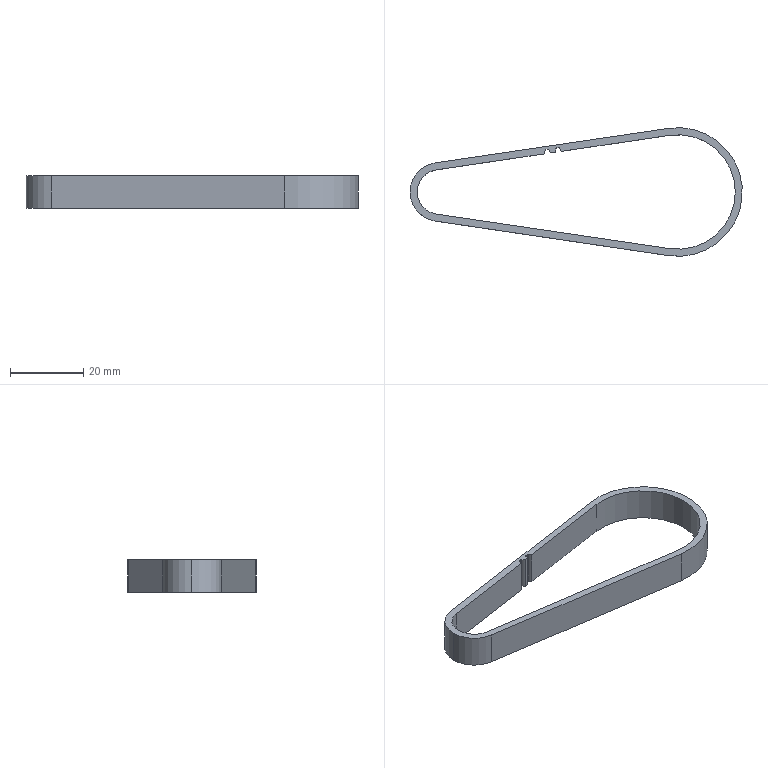Part | STEP file | Timing belt 210-3M-9mm wide_16-36 | 1 solid | 26 faces | box 90.97 x 35.218 x 9 mm | volume 3580 mm3 | cylinder 16 | plane 10 | commonest cylinder face diameters 0.6 x4 3.9 x4 0.2 x2 12.238 x2 16.118 x2 31.338 x1